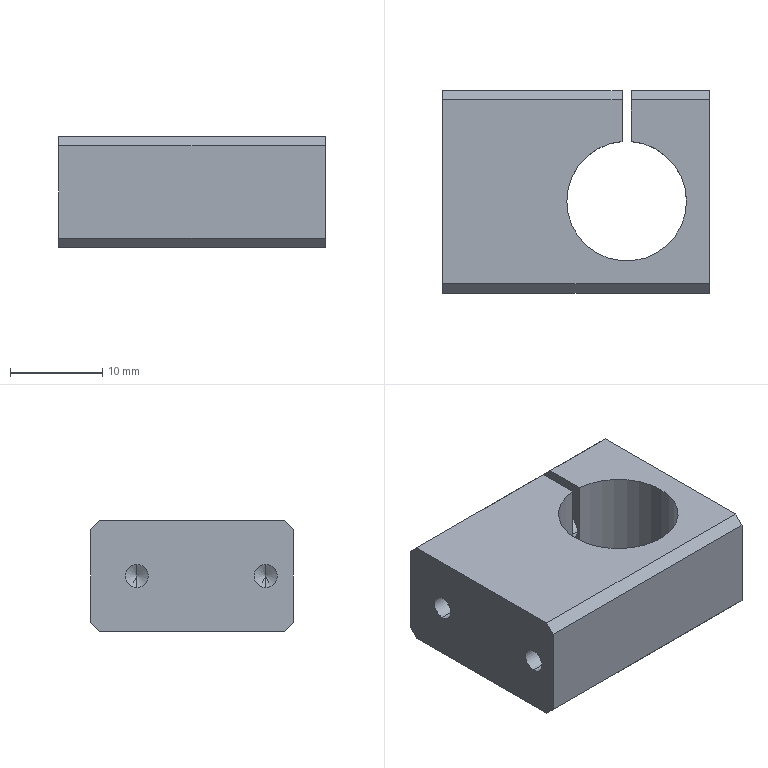NC program | NX | posted with a generic post | part box 29 x 22 x 12 mm
Whole program:
N10 G17 G21 G94 G90
(FLOOR_WALL_COPY_COPY , TOOL : D63)
N12 T03 M6
N14 G54
N16 G17 G0 G90 X48.999 Y0. B0. C0. S6500 M3
N18 G43 Z30. H3
N20 Z5.
N22 G94 G1 Z2. F1250.
N24 X45.999
N26 X-45.999
N28 X-48.999
N30 Z5.
N32 G0 Z30.
N34 X48.999
N36 Z4.
N38 G1 Z1.
N40 X45.999
N42 X-45.999
N44 X-48.999
N46 Z4.
N48 G0 Z30.
N50 X48.999
N52 Z3.
N54 G1 Z0.
N56 X45.999
N58 X-45.999
N60 X-48.999
N62 Z3.
N64 G0 Z30.
N66 M5
(11_COPY_COPY_COPY , TOOL : D6A45)
N68 T01 M6
N70 G54
N72 G17 G0 G90 X4.646 Y-2.745 B0. C0. S9500 M3
N74 G43 Z30. H1
N76 Z1.5
N78 G94 G1 Z-1.5 F1000.
N80 X5.346 Y-3.767
N82 G3 X5.887 Y-4.027 R0.6
N84 X5.113 Y-4.027 R-5.041
N86 G2 X5.498 Y-4.112 R1.432
N88 G1 X5.836 Y-4.032
N90 X5.887 Y-4.027
N92 G3 X6.374 Y-3.676 R0.6
N94 G1 X6.863 Y-2.592
N96 Z1.5
N98 G0 Z30.
N100 X-15.441 Y12.487
N102 Z1.5
N104 G1 Z-1.5
N106 X-15.02 Y11.759
N108 G3 X-14.501 Y11.459 R0.6
N110 G1 X14.501
N112 G2 X15.959 Y10.001 R1.458
N114 G1 Y-10.001
N116 G2 X14.501 Y-11.459 R1.458
N118 G1 X5.999
N120 G2 X5.502 Y-11.368 R1.42
N122 X5.001 Y-11.459 R1.464
N124 G1 X-14.501
N126 G2 X-15.959 Y-10.001 R1.458
N128 G1 Y10.001
N130 G2 X-14.501 Y11.459 R1.458
N132 G3 X-13.981 Y11.759 R0.6
N134 G1 X-13.461 Y12.659
N136 Z1.5
N138 G0 Z30.
N140 M5
N142 M2